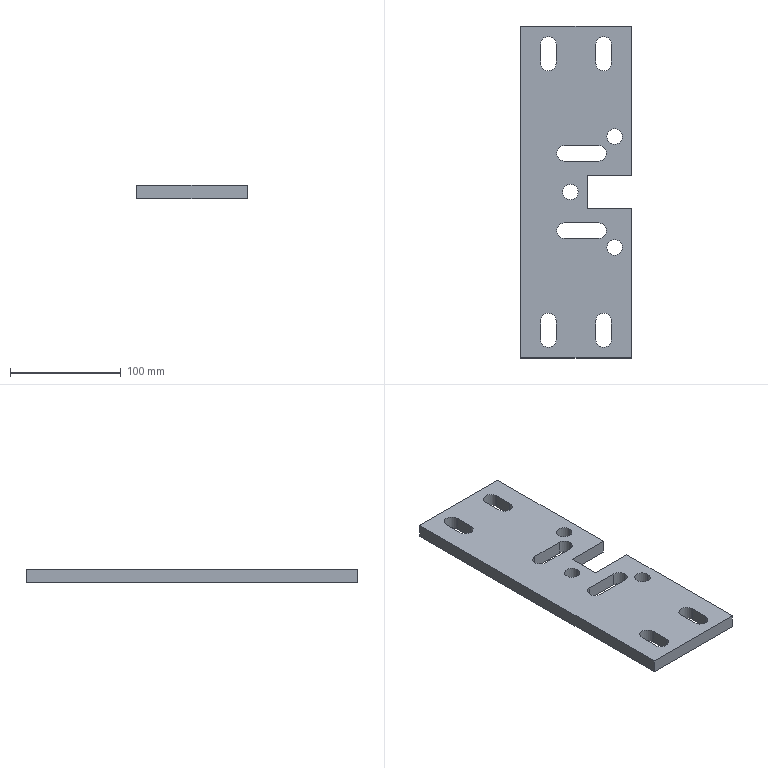Part | 1 solid | 42 faces | box 100 x 300 x 12 mm | volume 307135 mm3 | plane 22 | cylinder 20 | commonest cylinder face diameters 14 x20
STEP:
#1=CARTESIAN_POINT('',(28.,-50.,-12.));
#2=VERTEX_POINT('',#1);
#3=CARTESIAN_POINT('',(42.,-50.,-12.));
#4=VERTEX_POINT('',#3);
#5=CARTESIAN_POINT('',(35.,-50.,-12.));
#6=DIRECTION('',(0.,0.,1.));
#7=DIRECTION('',(1.,0.,0.));
#8=AXIS2_PLACEMENT_3D('',#5,#6,#7);
#9=CIRCLE('',#8,7.);
#10=EDGE_CURVE('',#2,#4,#9,.T.);
#11=ORIENTED_EDGE('',*,*,#10,.F.);
#12=CARTESIAN_POINT('',(28.,-50.,0.));
#13=VERTEX_POINT('',#12);
#14=CARTESIAN_POINT('',(28.,-50.,-12.));
#15=DIRECTION('',(0.,0.,1.));
#16=VECTOR('',#15,1000.);
#17=LINE('',#14,#16);
#18=EDGE_CURVE('',#2,#13,#17,.T.);
#19=ORIENTED_EDGE('',*,*,#18,.T.);
#20=CARTESIAN_POINT('',(42.,-50.,0.));
#21=VERTEX_POINT('',#20);
#22=CARTESIAN_POINT('',(35.,-50.,0.));
#23=DIRECTION('',(0.,0.,1.));
#24=DIRECTION('',(1.,0.,0.));
#25=AXIS2_PLACEMENT_3D('',#22,#23,#24);
#26=CIRCLE('',#25,7.);
#27=EDGE_CURVE('',#13,#21,#26,.T.);
#28=ORIENTED_EDGE('',*,*,#27,.T.);
#29=CARTESIAN_POINT('',(42.,-50.,-12.));
#30=DIRECTION('',(0.,0.,1.));
#31=VECTOR('',#30,1000.);
#32=LINE('',#29,#31);
#33=EDGE_CURVE('',#4,#21,#32,.T.);
#34=ORIENTED_EDGE('',*,*,#33,.F.);
#35=EDGE_LOOP('',(#11,#19,#28,#34));
#36=FACE_OUTER_BOUND('',#35,.T.);
#37=CARTESIAN_POINT('',(35.,-50.,-12.));
#38=DIRECTION('',(0.,0.,1.));
#39=DIRECTION('',(1.,0.,0.));
#40=AXIS2_PLACEMENT_3D('',#37,#38,#39);
#41=CYLINDRICAL_SURFACE('',#40,7.);
#42=ADVANCED_FACE('',(#36),#41,.F.);
#43=CARTESIAN_POINT('',(-12.,0.,-12.));
#44=VERTEX_POINT('',#43);
#45=CARTESIAN_POINT('',(2.,0.,-12.));
#46=VERTEX_POINT('',#45);
#47=CARTESIAN_POINT('',(-5.,0.,-12.));
#48=DIRECTION('',(0.,0.,1.));
#49=DIRECTION('',(1.,0.,0.));
#50=AXIS2_PLACEMENT_3D('',#47,#48,#49);
#51=CIRCLE('',#50,7.);
#52=EDGE_CURVE('',#44,#46,#51,.T.);
#53=ORIENTED_EDGE('',*,*,#52,.F.);
#54=CARTESIAN_POINT('',(-12.,0.,0.));
#55=VERTEX_POINT('',#54);
#56=CARTESIAN_POINT('',(-12.,0.,-12.));
#57=DIRECTION('',(0.,0.,1.));
#58=VECTOR('',#57,1000.);
#59=LINE('',#56,#58);
#60=EDGE_CURVE('',#44,#55,#59,.T.);
#61=ORIENTED_EDGE('',*,*,#60,.T.);
#62=CARTESIAN_POINT('',(2.,0.,0.));
#63=VERTEX_POINT('',#62);
#64=CARTESIAN_POINT('',(-5.,0.,0.));
#65=DIRECTION('',(0.,0.,1.));
#66=DIRECTION('',(1.,0.,0.));
#67=AXIS2_PLACEMENT_3D('',#64,#65,#66);
#68=CIRCLE('',#67,7.);
#69=EDGE_CURVE('',#55,#63,#68,.T.);
#70=ORIENTED_EDGE('',*,*,#69,.T.);
#71=CARTESIAN_POINT('',(2.,0.,-12.));
#72=DIRECTION('',(0.,0.,1.));
#73=VECTOR('',#72,1000.);
#74=LINE('',#71,#73);
#75=EDGE_CURVE('',#46,#63,#74,.T.);
#76=ORIENTED_EDGE('',*,*,#75,.F.);
#77=EDGE_LOOP('',(#53,#61,#70,#76));
#78=FACE_OUTER_BOUND('',#77,.T.);
#79=CARTESIAN_POINT('',(-5.,0.,-12.));
#80=DIRECTION('',(0.,0.,1.));
#81=DIRECTION('',(1.,0.,0.));
#82=AXIS2_PLACEMENT_3D('',#79,#80,#81);
#83=CYLINDRICAL_SURFACE('',#82,7.);
#84=ADVANCED_FACE('',(#78),#83,.F.);
#85=CARTESIAN_POINT('',(28.,50.,-12.));
#86=VERTEX_POINT('',#85);
#87=CARTESIAN_POINT('',(42.,50.,-12.));
#88=VERTEX_POINT('',#87);
#89=CARTESIAN_POINT('',(35.,50.,-12.));
#90=DIRECTION('',(0.,0.,1.));
#91=DIRECTION('',(-1.,0.,0.));
#92=AXIS2_PLACEMENT_3D('',#89,#90,#91);
#93=CIRCLE('',#92,7.);
#94=EDGE_CURVE('',#86,#88,#93,.T.);
#95=ORIENTED_EDGE('',*,*,#94,.F.);
#96=CARTESIAN_POINT('',(28.,50.,0.));
#97=VERTEX_POINT('',#96);
#98=CARTESIAN_POINT('',(28.,50.,-12.));
#99=DIRECTION('',(0.,0.,1.));
#100=VECTOR('',#99,1000.);
#101=LINE('',#98,#100);
#102=EDGE_CURVE('',#86,#97,#101,.T.);
#103=ORIENTED_EDGE('',*,*,#102,.T.);
#104=CARTESIAN_POINT('',(42.,50.,0.));
#105=VERTEX_POINT('',#104);
#106=CARTESIAN_POINT('',(35.,50.,0.));
#107=DIRECTION('',(0.,0.,1.));
#108=DIRECTION('',(1.,0.,0.));
#109=AXIS2_PLACEMENT_3D('',#106,#107,#108);
#110=CIRCLE('',#109,7.);
#111=EDGE_CURVE('',#97,#105,#110,.T.);
#112=ORIENTED_EDGE('',*,*,#111,.T.);
#113=CARTESIAN_POINT('',(42.,50.,-12.));
#114=DIRECTION('',(0.,0.,1.));
#115=VECTOR('',#114,1000.);
#116=LINE('',#113,#115);
#117=EDGE_CURVE('',#88,#105,#116,.T.);
#118=ORIENTED_EDGE('',*,*,#117,.F.);
#119=EDGE_LOOP('',(#95,#103,#112,#118));
#120=FACE_OUTER_BOUND('',#119,.T.);
#121=CARTESIAN_POINT('',(35.,50.,-12.));
#122=DIRECTION('',(0.,0.,1.));
#123=DIRECTION('',(1.,0.,0.));
#124=AXIS2_PLACEMENT_3D('',#121,#122,#123);
#125=CYLINDRICAL_SURFACE('',#124,7.);
#126=ADVANCED_FACE('',(#120),#125,.F.);
#127=CARTESIAN_POINT('',(27.5,-35.,-12.));
#128=VERTEX_POINT('',#127);
#129=CARTESIAN_POINT('',(20.5,-28.,-12.));
#130=VERTEX_POINT('',#129);
#131=CARTESIAN_POINT('',(20.5,-35.,-12.));
#132=DIRECTION('',(0.,0.,1.));
#133=DIRECTION('',(1.,0.,0.));
#134=AXIS2_PLACEMENT_3D('',#131,#132,#133);
#135=CIRCLE('',#134,7.);
#136=EDGE_CURVE('',#128,#130,#135,.T.);
#137=ORIENTED_EDGE('',*,*,#136,.F.);
#138=CARTESIAN_POINT('',(27.5,-35.,0.));
#139=VERTEX_POINT('',#138);
#140=CARTESIAN_POINT('',(27.5,-35.,-12.));
#141=DIRECTION('',(0.,0.,1.));
#142=VECTOR('',#141,1000.);
#143=LINE('',#140,#142);
#144=EDGE_CURVE('',#128,#139,#143,.T.);
#145=ORIENTED_EDGE('',*,*,#144,.T.);
#146=CARTESIAN_POINT('',(20.5,-28.,0.));
#147=VERTEX_POINT('',#146);
#148=CARTESIAN_POINT('',(20.5,-35.,0.));
#149=DIRECTION('',(0.,0.,1.));
#150=DIRECTION('',(1.,0.,0.));
#151=AXIS2_PLACEMENT_3D('',#148,#149,#150);
#152=CIRCLE('',#151,7.);
#153=EDGE_CURVE('',#139,#147,#152,.T.);
#154=ORIENTED_EDGE('',*,*,#153,.T.);
#155=CARTESIAN_POINT('',(20.5,-28.,-12.));
#156=DIRECTION('',(0.,0.,1.));
#157=VECTOR('',#156,1000.);
#158=LINE('',#155,#157);
#159=EDGE_CURVE('',#130,#147,#158,.T.);
#160=ORIENTED_EDGE('',*,*,#159,.F.);
#161=EDGE_LOOP('',(#137,#145,#154,#160));
#162=FACE_OUTER_BOUND('',#161,.T.);
#163=CARTESIAN_POINT('',(20.5,-35.,-12.));
#164=DIRECTION('',(0.,0.,1.));
#165=DIRECTION('',(1.,0.,0.));
#166=AXIS2_PLACEMENT_3D('',#163,#164,#165);
#167=CYLINDRICAL_SURFACE('',#166,7.);
#168=ADVANCED_FACE('',(#162),#167,.F.);
#169=CARTESIAN_POINT('',(27.5,35.,-12.));
#170=VERTEX_POINT('',#169);
#171=CARTESIAN_POINT('',(20.5,42.,-12.));
#172=VERTEX_POINT('',#171);
#173=CARTESIAN_POINT('',(20.5,35.,-12.));
#174=DIRECTION('',(0.,0.,1.));
#175=DIRECTION('',(-1.,0.,0.));
#176=AXIS2_PLACEMENT_3D('',#173,#174,#175);
#177=CIRCLE('',#176,7.);
#178=EDGE_CURVE('',#170,#172,#177,.T.);
#179=ORIENTED_EDGE('',*,*,#178,.F.);
#180=CARTESIAN_POINT('',(27.5,35.,0.));
#181=VERTEX_POINT('',#180);
#182=CARTESIAN_POINT('',(27.5,35.,-12.));
#183=DIRECTION('',(0.,0.,1.));
#184=VECTOR('',#183,1000.);
#185=LINE('',#182,#184);
#186=EDGE_CURVE('',#170,#181,#185,.T.);
#187=ORIENTED_EDGE('',*,*,#186,.T.);
#188=CARTESIAN_POINT('',(20.5,42.,0.));
#189=VERTEX_POINT('',#188);
#190=CARTESIAN_POINT('',(20.5,35.,0.));
#191=DIRECTION('',(0.,0.,1.));
#192=DIRECTION('',(1.,0.,0.));
#193=AXIS2_PLACEMENT_3D('',#190,#191,#192);
#194=CIRCLE('',#193,7.);
#195=EDGE_CURVE('',#181,#189,#194,.T.);
#196=ORIENTED_EDGE('',*,*,#195,.T.);
#197=CARTESIAN_POINT('',(20.5,42.,-12.));
#198=DIRECTION('',(0.,0.,1.));
#199=VECTOR('',#198,1000.);
#200=LINE('',#197,#199);
#201=EDGE_CURVE('',#172,#189,#200,.T.);
#202=ORIENTED_EDGE('',*,*,#201,.F.);
#203=EDGE_LOOP('',(#179,#187,#196,#202));
#204=FACE_OUTER_BOUND('',#203,.T.);
#205=CARTESIAN_POINT('',(20.5,35.,-12.));
#206=DIRECTION('',(0.,0.,1.));
#207=DIRECTION('',(1.,0.,0.));
#208=AXIS2_PLACEMENT_3D('',#205,#206,#207);
#209=CYLINDRICAL_SURFACE('',#208,7.);
#210=ADVANCED_FACE('',(#204),#209,.F.);
#211=CARTESIAN_POINT('',(50.,-15.,0.));
#212=VERTEX_POINT('',#211);
#213=CARTESIAN_POINT('',(50.,-15.,-12.));
#214=VERTEX_POINT('',#213);
#215=CARTESIAN_POINT('',(50.,-15.,-12.));
#216=DIRECTION('',(0.,0.,-1.));
#217=VECTOR('',#216,1000.);
#218=LINE('',#215,#217);
#219=EDGE_CURVE('',#212,#214,#218,.T.);
#220=ORIENTED_EDGE('',*,*,#219,.F.);
#221=CARTESIAN_POINT('',(50.,-150.,0.));
#222=VERTEX_POINT('',#221);
#223=CARTESIAN_POINT('',(50.,150.,0.));
#224=DIRECTION('',(0.,1.,0.));
#225=VECTOR('',#224,1000.);
#226=LINE('',#223,#225);
#227=EDGE_CURVE('',#222,#212,#226,.T.);
#228=ORIENTED_EDGE('',*,*,#227,.F.);
#229=CARTESIAN_POINT('',(50.,-150.,-12.));
#230=VERTEX_POINT('',#229);
#231=CARTESIAN_POINT('',(50.,-150.,-12.));
#232=DIRECTION('',(0.,0.,1.));
#233=VECTOR('',#232,1000.);
#234=LINE('',#231,#233);
#235=EDGE_CURVE('',#230,#222,#234,.T.);
#236=ORIENTED_EDGE('',*,*,#235,.F.);
#237=CARTESIAN_POINT('',(50.,150.,-12.));
#238=DIRECTION('',(0.,1.,0.));
#239=VECTOR('',#238,1000.);
#240=LINE('',#237,#239);
#241=EDGE_CURVE('',#230,#214,#240,.T.);
#242=ORIENTED_EDGE('',*,*,#241,.T.);
#243=EDGE_LOOP('',(#220,#228,#236,#242));
#244=FACE_OUTER_BOUND('',#243,.T.);
#245=CARTESIAN_POINT('',(50.,150.,-12.));
#246=DIRECTION('',(1.,0.,0.));
#247=DIRECTION('',(0.,1.,0.));
#248=AXIS2_PLACEMENT_3D('',#245,#246,#247);
#249=PLANE('',#248);
#250=ADVANCED_FACE('',(#244),#249,.T.);
#251=CARTESIAN_POINT('',(50.,15.,-12.));
#252=VERTEX_POINT('',#251);
#253=CARTESIAN_POINT('',(50.,15.,0.));
#254=VERTEX_POINT('',#253);
#255=CARTESIAN_POINT('',(50.,15.,-12.));
#256=DIRECTION('',(0.,0.,1.));
#257=VECTOR('',#256,1000.);
#258=LINE('',#255,#257);
#259=EDGE_CURVE('',#252,#254,#258,.T.);
#260=ORIENTED_EDGE('',*,*,#259,.F.);
#261=CARTESIAN_POINT('',(50.,150.,-12.));
#262=VERTEX_POINT('',#261);
#263=CARTESIAN_POINT('',(50.,150.,-12.));
#264=DIRECTION('',(0.,1.,0.));
#265=VECTOR('',#264,1000.);
#266=LINE('',#263,#265);
#267=EDGE_CURVE('',#252,#262,#266,.T.);
#268=ORIENTED_EDGE('',*,*,#267,.T.);
#269=CARTESIAN_POINT('',(50.,150.,0.));
#270=VERTEX_POINT('',#269);
#271=CARTESIAN_POINT('',(50.,150.,-12.));
#272=DIRECTION('',(0.,0.,1.));
#273=VECTOR('',#272,1000.);
#274=LINE('',#271,#273);
#275=EDGE_CURVE('',#262,#270,#274,.T.);
#276=ORIENTED_EDGE('',*,*,#275,.T.);
#277=CARTESIAN_POINT('',(50.,150.,0.));
#278=DIRECTION('',(0.,1.,0.));
#279=VECTOR('',#278,1000.);
#280=LINE('',#277,#279);
#281=EDGE_CURVE('',#254,#270,#280,.T.);
#282=ORIENTED_EDGE('',*,*,#281,.F.);
#283=EDGE_LOOP('',(#260,#268,#276,#282));
#284=FACE_OUTER_BOUND('',#283,.T.);
#285=CARTESIAN_POINT('',(50.,150.,-12.));
#286=DIRECTION('',(1.,0.,0.));
#287=DIRECTION('',(0.,1.,0.));
#288=AXIS2_PLACEMENT_3D('',#285,#286,#287);
#289=PLANE('',#288);
#290=ADVANCED_FACE('',(#284),#289,.T.);
#291=CARTESIAN_POINT('',(-50.,-150.,0.));
#292=VERTEX_POINT('',#291);
#293=CARTESIAN_POINT('',(-50.,-150.,0.));
#294=DIRECTION('',(1.,0.,0.));
#295=VECTOR('',#294,1000.);
#296=LINE('',#293,#295);
#297=EDGE_CURVE('',#292,#222,#296,.T.);
#298=ORIENTED_EDGE('',*,*,#297,.F.);
#299=CARTESIAN_POINT('',(-50.,-150.,-12.));
#300=VERTEX_POINT('',#299);
#301=CARTESIAN_POINT('',(-50.,-150.,-12.));
#302=DIRECTION('',(0.,0.,1.));
#303=VECTOR('',#302,1000.);
#304=LINE('',#301,#303);
#305=EDGE_CURVE('',#300,#292,#304,.T.);
#306=ORIENTED_EDGE('',*,*,#305,.F.);
#307=CARTESIAN_POINT('',(-50.,-150.,-12.));
#308=DIRECTION('',(1.,0.,0.));
#309=VECTOR('',#308,1000.);
#310=LINE('',#307,#309);
#311=EDGE_CURVE('',#300,#230,#310,.T.);
#312=ORIENTED_EDGE('',*,*,#311,.T.);
#313=ORIENTED_EDGE('',*,*,#235,.T.);
#314=EDGE_LOOP('',(#298,#306,#312,#313));
#315=FACE_OUTER_BOUND('',#314,.T.);
#316=CARTESIAN_POINT('',(-50.,-150.,-12.));
#317=DIRECTION('',(0.,-1.,0.));
#318=DIRECTION('',(0.,0.,-1.));
#319=AXIS2_PLACEMENT_3D('',#316,#317,#318);
#320=PLANE('',#319);
#321=ADVANCED_FACE('',(#315),#320,.T.);
#322=CARTESIAN_POINT('',(-50.,150.,0.));
#323=VERTEX_POINT('',#322);
#324=CARTESIAN_POINT('',(-50.,150.,0.));
#325=DIRECTION('',(0.,-1.,0.));
#326=VECTOR('',#325,1000.);
#327=LINE('',#324,#326);
#328=EDGE_CURVE('',#323,#292,#327,.T.);
#329=ORIENTED_EDGE('',*,*,#328,.F.);
#330=CARTESIAN_POINT('',(-50.,150.,-12.));
#331=VERTEX_POINT('',#330);
#332=CARTESIAN_POINT('',(-50.,150.,-12.));
#333=DIRECTION('',(0.,0.,1.));
#334=VECTOR('',#333,1000.);
#335=LINE('',#332,#334);
#336=EDGE_CURVE('',#331,#323,#335,.T.);
#337=ORIENTED_EDGE('',*,*,#336,.F.);
#338=CARTESIAN_POINT('',(-50.,150.,-12.));
#339=DIRECTION('',(0.,-1.,0.));
#340=VECTOR('',#339,1000.);
#341=LINE('',#338,#340);
#342=EDGE_CURVE('',#331,#300,#341,.T.);
#343=ORIENTED_EDGE('',*,*,#342,.T.);
#344=ORIENTED_EDGE('',*,*,#305,.T.);
#345=EDGE_LOOP('',(#329,#337,#343,#344));
#346=FACE_OUTER_BOUND('',#345,.T.);
#347=CARTESIAN_POINT('',(-50.,150.,-12.));
#348=DIRECTION('',(-1.,0.,0.));
#349=DIRECTION('',(0.,-1.,0.));
#350=AXIS2_PLACEMENT_3D('',#347,#348,#349);
#351=PLANE('',#350);
#352=ADVANCED_FACE('',(#346),#351,.T.);
#353=CARTESIAN_POINT('',(-50.,150.,0.));
#354=DIRECTION('',(-1.,0.,0.));
#355=VECTOR('',#354,1000.);
#356=LINE('',#353,#355);
#357=EDGE_CURVE('',#270,#323,#356,.T.);
#358=ORIENTED_EDGE('',*,*,#357,.F.);
#359=ORIENTED_EDGE('',*,*,#275,.F.);
#360=CARTESIAN_POINT('',(-50.,150.,-12.));
#361=DIRECTION('',(-1.,0.,0.));
#362=VECTOR('',#361,1000.);
#363=LINE('',#360,#362);
#364=EDGE_CURVE('',#262,#331,#363,.T.);
#365=ORIENTED_EDGE('',*,*,#364,.T.);
#366=ORIENTED_EDGE('',*,*,#336,.T.);
#367=EDGE_LOOP('',(#358,#359,#365,#366));
#368=FACE_OUTER_BOUND('',#367,.T.);
#369=CARTESIAN_POINT('',(-50.,150.,-12.));
#370=DIRECTION('',(0.,1.,0.));
#371=DIRECTION('',(0.,0.,1.));
#372=AXIS2_PLACEMENT_3D('',#369,#370,#371);
#373=PLANE('',#372);
#374=ADVANCED_FACE('',(#368),#373,.T.);
#375=CARTESIAN_POINT('',(35.,-50.,-12.));
#376=DIRECTION('',(0.,0.,1.));
#377=DIRECTION('',(1.,0.,0.));
#378=AXIS2_PLACEMENT_3D('',#375,#376,#377);
#379=CIRCLE('',#378,7.);
#380=EDGE_CURVE('',#4,#2,#379,.T.);
#381=ORIENTED_EDGE('',*,*,#380,.T.);
#382=ORIENTED_EDGE('',*,*,#10,.T.);
#383=EDGE_LOOP('',(#381,#382));
#384=FACE_BOUND('',#383,.T.);
#385=CARTESIAN_POINT('',(-5.,0.,-12.));
#386=DIRECTION('',(0.,0.,1.));
#387=DIRECTION('',(1.,0.,0.));
#388=AXIS2_PLACEMENT_3D('',#385,#386,#387);
#389=CIRCLE('',#388,7.);
#390=EDGE_CURVE('',#46,#44,#389,.T.);
#391=ORIENTED_EDGE('',*,*,#390,.T.);
#392=ORIENTED_EDGE('',*,*,#52,.T.);
#393=EDGE_LOOP('',(#391,#392));
#394=FACE_BOUND('',#393,.T.);
#395=CARTESIAN_POINT('',(35.,50.,-12.));
#396=DIRECTION('',(0.,0.,1.));
#397=DIRECTION('',(-1.,0.,0.));
#398=AXIS2_PLACEMENT_3D('',#395,#396,#397);
#399=CIRCLE('',#398,7.);
#400=EDGE_CURVE('',#88,#86,#399,.T.);
#401=ORIENTED_EDGE('',*,*,#400,.T.);
#402=ORIENTED_EDGE('',*,*,#94,.T.);
#403=EDGE_LOOP('',(#401,#402));
#404=FACE_BOUND('',#403,.T.);
#405=CARTESIAN_POINT('',(-10.5,-28.,-12.));
#406=VERTEX_POINT('',#405);
#407=CARTESIAN_POINT('',(-10.5,-28.,-12.));
#408=DIRECTION('',(-1.,0.,0.));
#409=VECTOR('',#408,1000.);
#410=LINE('',#407,#409);
#411=EDGE_CURVE('',#130,#406,#410,.T.);
#412=ORIENTED_EDGE('',*,*,#411,.T.);
#413=CARTESIAN_POINT('',(-10.5,-42.,-12.));
#414=VERTEX_POINT('',#413);
#415=CARTESIAN_POINT('',(-10.5,-35.,-12.));
#416=DIRECTION('',(0.,0.,1.));
#417=DIRECTION('',(1.,0.,0.));
#418=AXIS2_PLACEMENT_3D('',#415,#416,#417);
#419=CIRCLE('',#418,7.);
#420=EDGE_CURVE('',#406,#414,#419,.T.);
#421=ORIENTED_EDGE('',*,*,#420,.T.);
#422=CARTESIAN_POINT('',(20.5,-42.,-12.));
#423=VERTEX_POINT('',#422);
#424=CARTESIAN_POINT('',(-10.5,-42.,-12.));
#425=DIRECTION('',(1.,0.,0.));
#426=VECTOR('',#425,1000.);
#427=LINE('',#424,#426);
#428=EDGE_CURVE('',#414,#423,#427,.T.);
#429=ORIENTED_EDGE('',*,*,#428,.T.);
#430=CARTESIAN_POINT('',(20.5,-35.,-12.));
#431=DIRECTION('',(0.,0.,1.));
#432=DIRECTION('',(1.,0.,0.));
#433=AXIS2_PLACEMENT_3D('',#430,#431,#432);
#434=CIRCLE('',#433,7.);
#435=EDGE_CURVE('',#423,#128,#434,.T.);
#436=ORIENTED_EDGE('',*,*,#435,.T.);
#437=ORIENTED_EDGE('',*,*,#136,.T.);
#438=EDGE_LOOP('',(#412,#421,#429,#436,#437));
#439=FACE_BOUND('',#438,.T.);
#440=CARTESIAN_POINT('',(-18.,116.5,-12.));
#441=VERTEX_POINT('',#440);
#442=CARTESIAN_POINT('',(-18.,133.5,-12.));
#443=VERTEX_POINT('',#442);
#444=CARTESIAN_POINT('',(-18.,133.5,-12.));
#445=DIRECTION('',(0.,1.,0.));
#446=VECTOR('',#445,1000.);
#447=LINE('',#444,#446);
#448=EDGE_CURVE('',#441,#443,#447,.T.);
#449=ORIENTED_EDGE('',*,*,#448,.T.);
#450=CARTESIAN_POINT('',(-32.,133.5,-12.));
#451=VERTEX_POINT('',#450);
#452=CARTESIAN_POINT('',(-25.,133.5,-12.));
#453=DIRECTION('',(0.,0.,1.));
#454=DIRECTION('',(-1.,0.,0.));
#455=AXIS2_PLACEMENT_3D('',#452,#453,#454);
#456=CIRCLE('',#455,7.);
#457=EDGE_CURVE('',#443,#451,#456,.T.);
#458=ORIENTED_EDGE('',*,*,#457,.T.);
#459=CARTESIAN_POINT('',(-32.,116.5,-12.));
#460=VERTEX_POINT('',#459);
#461=CARTESIAN_POINT('',(-32.,133.5,-12.));
#462=DIRECTION('',(0.,-1.,0.));
#463=VECTOR('',#462,1000.);
#464=LINE('',#461,#463);
#465=EDGE_CURVE('',#451,#460,#464,.T.);
#466=ORIENTED_EDGE('',*,*,#465,.T.);
#467=CARTESIAN_POINT('',(-25.,116.5,-12.));
#468=DIRECTION('',(0.,0.,1.));
#469=DIRECTION('',(-1.,0.,0.));
#470=AXIS2_PLACEMENT_3D('',#467,#468,#469);
#471=CIRCLE('',#470,7.);
#472=EDGE_CURVE('',#460,#441,#471,.T.);
#473=ORIENTED_EDGE('',*,*,#472,.T.);
#474=EDGE_LOOP('',(#449,#458,#466,#473));
#475=FACE_BOUND('',#474,.T.);
#476=CARTESIAN_POINT('',(32.,116.5,-12.));
#477=VERTEX_POINT('',#476);
#478=CARTESIAN_POINT('',(32.,133.5,-12.));
#479=VERTEX_POINT('',#478);
#480=CARTESIAN_POINT('',(32.,133.5,-12.));
#481=DIRECTION('',(0.,1.,0.));
#482=VECTOR('',#481,1000.);
#483=LINE('',#480,#482);
#484=EDGE_CURVE('',#477,#479,#483,.T.);
#485=ORIENTED_EDGE('',*,*,#484,.T.);
#486=CARTESIAN_POINT('',(18.,133.5,-12.));
#487=VERTEX_POINT('',#486);
#488=CARTESIAN_POINT('',(25.,133.5,-12.));
#489=DIRECTION('',(0.,0.,1.));
#490=DIRECTION('',(-1.,0.,0.));
#491=AXIS2_PLACEMENT_3D('',#488,#489,#490);
#492=CIRCLE('',#491,7.);
#493=EDGE_CURVE('',#479,#487,#492,.T.);
#494=ORIENTED_EDGE('',*,*,#493,.T.);
#495=CARTESIAN_POINT('',(18.,116.5,-12.));
#496=VERTEX_POINT('',#495);
#497=CARTESIAN_POINT('',(18.,133.5,-12.));
#498=DIRECTION('',(0.,-1.,0.));
#499=VECTOR('',#498,1000.);
#500=LINE('',#497,#499);
#501=EDGE_CURVE('',#487,#496,#500,.T.);
#502=ORIENTED_EDGE('',*,*,#501,.T.);
#503=CARTESIAN_POINT('',(25.,116.5,-12.));
#504=DIRECTION('',(0.,0.,1.));
#505=DIRECTION('',(-1.,0.,0.));
#506=AXIS2_PLACEMENT_3D('',#503,#504,#505);
#507=CIRCLE('',#506,7.);
#508=EDGE_CURVE('',#496,#477,#507,.T.);
#509=ORIENTED_EDGE('',*,*,#508,.T.);
#510=EDGE_LOOP('',(#485,#494,#502,#509));
#511=FACE_BOUND('',#510,.T.);
#512=CARTESIAN_POINT('',(18.,-116.5,-12.));
#513=VERTEX_POINT('',#512);
#514=CARTESIAN_POINT('',(18.,-133.5,-12.));
#515=VERTEX_POINT('',#514);
#516=CARTESIAN_POINT('',(18.,-133.5,-12.));
#517=DIRECTION('',(0.,-1.,0.));
#518=VECTOR('',#517,1000.);
#519=LINE('',#516,#518);
#520=EDGE_CURVE('',#513,#515,#519,.T.);
#521=ORIENTED_EDGE('',*,*,#520,.T.);
#522=CARTESIAN_POINT('',(32.,-133.5,-12.));
#523=VERTEX_POINT('',#522);
#524=CARTESIAN_POINT('',(25.,-133.5,-12.));
#525=DIRECTION('',(0.,0.,1.));
#526=DIRECTION('',(1.,0.,0.));
#527=AXIS2_PLACEMENT_3D('',#524,#525,#526);
#528=CIRCLE('',#527,7.);
#529=EDGE_CURVE('',#515,#523,#528,.T.);
#530=ORIENTED_EDGE('',*,*,#529,.T.);
#531=CARTESIAN_POINT('',(32.,-116.5,-12.));
#532=VERTEX_POINT('',#531);
#533=CARTESIAN_POINT('',(32.,-133.5,-12.));
#534=DIRECTION('',(0.,1.,0.));
#535=VECTOR('',#534,1000.);
#536=LINE('',#533,#535);
#537=EDGE_CURVE('',#523,#532,#536,.T.);
#538=ORIENTED_EDGE('',*,*,#537,.T.);
#539=CARTESIAN_POINT('',(25.,-116.5,-12.));
#540=DIRECTION('',(0.,0.,1.));
#541=DIRECTION('',(1.,0.,0.));
#542=AXIS2_PLACEMENT_3D('',#539,#540,#541);
#543=CIRCLE('',#542,7.);
#544=EDGE_CURVE('',#532,#513,#543,.T.);
#545=ORIENTED_EDGE('',*,*,#544,.T.);
#546=EDGE_LOOP('',(#521,#530,#538,#545));
#547=FACE_BOUND('',#546,.T.);
#548=CARTESIAN_POINT('',(-32.,-116.5,-12.));
#549=VERTEX_POINT('',#548);
#550=CARTESIAN_POINT('',(-32.,-133.5,-12.));
#551=VERTEX_POINT('',#550);
#552=CARTESIAN_POINT('',(-32.,-133.5,-12.));
#553=DIRECTION('',(0.,-1.,0.));
#554=VECTOR('',#553,1000.);
#555=LINE('',#552,#554);
#556=EDGE_CURVE('',#549,#551,#555,.T.);
#557=ORIENTED_EDGE('',*,*,#556,.T.);
#558=CARTESIAN_POINT('',(-18.,-133.5,-12.));
#559=VERTEX_POINT('',#558);
#560=CARTESIAN_POINT('',(-25.,-133.5,-12.));
#561=DIRECTION('',(0.,0.,1.));
#562=DIRECTION('',(1.,0.,0.));
#563=AXIS2_PLACEMENT_3D('',#560,#561,#562);
#564=CIRCLE('',#563,7.);
#565=EDGE_CURVE('',#551,#559,#564,.T.);
#566=ORIENTED_EDGE('',*,*,#565,.T.);
#567=CARTESIAN_POINT('',(-18.,-116.5,-12.));
#568=VERTEX_POINT('',#567);
#569=CARTESIAN_POINT('',(-18.,-133.5,-12.));
#570=DIRECTION('',(0.,1.,0.));
#571=VECTOR('',#570,1000.);
#572=LINE('',#569,#571);
#573=EDGE_CURVE('',#559,#568,#572,.T.);
#574=ORIENTED_EDGE('',*,*,#573,.T.);
#575=CARTESIAN_POINT('',(-25.,-116.5,-12.));
#576=DIRECTION('',(0.,0.,1.));
#577=DIRECTION('',(1.,0.,0.));
#578=AXIS2_PLACEMENT_3D('',#575,#576,#577);
#579=CIRCLE('',#578,7.);
#580=EDGE_CURVE('',#568,#549,#579,.T.);
#581=ORIENTED_EDGE('',*,*,#580,.T.);
#582=EDGE_LOOP('',(#557,#566,#574,#581));
#583=FACE_BOUND('',#582,.T.);
#584=CARTESIAN_POINT('',(-10.5,42.,-12.));
#585=VERTEX_POINT('',#584);
#586=CARTESIAN_POINT('',(-10.5,42.,-12.));
#587=DIRECTION('',(-1.,0.,0.));
#588=VECTOR('',#587,1000.);
#589=LINE('',#586,#588);
#590=EDGE_CURVE('',#172,#585,#589,.T.);
#591=ORIENTED_EDGE('',*,*,#590,.T.);
#592=CARTESIAN_POINT('',(-10.5,28.,-12.));
#593=VERTEX_POINT('',#592);
#594=CARTESIAN_POINT('',(-10.5,35.,-12.));
#595=DIRECTION('',(0.,0.,1.));
#596=DIRECTION('',(-1.,0.,0.));
#597=AXIS2_PLACEMENT_3D('',#594,#595,#596);
#598=CIRCLE('',#597,7.);
#599=EDGE_CURVE('',#585,#593,#598,.T.);
#600=ORIENTED_EDGE('',*,*,#599,.T.);
#601=CARTESIAN_POINT('',(20.5,28.,-12.));
#602=VERTEX_POINT('',#601);
#603=CARTESIAN_POINT('',(-10.5,28.,-12.));
#604=DIRECTION('',(1.,0.,0.));
#605=VECTOR('',#604,1000.);
#606=LINE('',#603,#605);
#607=EDGE_CURVE('',#593,#602,#606,.T.);
#608=ORIENTED_EDGE('',*,*,#607,.T.);
#609=CARTESIAN_POINT('',(20.5,35.,-12.));
#610=DIRECTION('',(0.,0.,1.));
#611=DIRECTION('',(-1.,0.,0.));
#612=AXIS2_PLACEMENT_3D('',#609,#610,#611);
#613=CIRCLE('',#612,7.);
#614=EDGE_CURVE('',#602,#170,#613,.T.);
#615=ORIENTED_EDGE('',*,*,#614,.T.);
#616=ORIENTED_EDGE('',*,*,#178,.T.);
#617=EDGE_LOOP('',(#591,#600,#608,#615,#616));
#618=FACE_BOUND('',#617,.T.);
#619=CARTESIAN_POINT('',(10.,15.,-12.));
#620=VERTEX_POINT('',#619);
#621=CARTESIAN_POINT('',(10.,-15.,-12.));
#622=VERTEX_POINT('',#621);
#623=CARTESIAN_POINT('',(10.,-15.,-12.));
#624=DIRECTION('',(0.,-1.,0.));
#625=VECTOR('',#624,1000.);
#626=LINE('',#623,#625);
#627=EDGE_CURVE('',#620,#622,#626,.T.);
#628=ORIENTED_EDGE('',*,*,#627,.T.);
#629=CARTESIAN_POINT('',(10.,-15.,-12.));
#630=DIRECTION('',(1.,0.,0.));
#631=VECTOR('',#630,1000.);
#632=LINE('',#629,#631);
#633=EDGE_CURVE('',#622,#214,#632,.T.);
#634=ORIENTED_EDGE('',*,*,#633,.T.);
#635=ORIENTED_EDGE('',*,*,#241,.F.);
#636=ORIENTED_EDGE('',*,*,#311,.F.);
#637=ORIENTED_EDGE('',*,*,#342,.F.);
#638=ORIENTED_EDGE('',*,*,#364,.F.);
#639=ORIENTED_EDGE('',*,*,#267,.F.);
#640=CARTESIAN_POINT('',(10.,15.,-12.));
#641=DIRECTION('',(-1.,0.,0.));
#642=VECTOR('',#641,1000.);
#643=LINE('',#640,#642);
#644=EDGE_CURVE('',#252,#620,#643,.T.);
#645=ORIENTED_EDGE('',*,*,#644,.T.);
#646=EDGE_LOOP('',(#628,#634,#635,#636,#637,#638,#639,#645));
#647=FACE_OUTER_BOUND('',#646,.T.);
#648=CARTESIAN_POINT('',(0.,0.,-12.));
#649=DIRECTION('',(0.,0.,1.));
#650=DIRECTION('',(1.,0.,0.));
#651=AXIS2_PLACEMENT_3D('',#648,#649,#650);
#652=PLANE('',#651);
#653=ADVANCED_FACE('',(#384,#394,#404,#439,#475,#511,#547,#583,#618,#647),#652,.F.);
#654=CARTESIAN_POINT('',(35.,-50.,0.));
#655=DIRECTION('',(0.,0.,1.));
#656=DIRECTION('',(1.,0.,0.));
#657=AXIS2_PLACEMENT_3D('',#654,#655,#656);
#658=CIRCLE('',#657,7.);
#659=EDGE_CURVE('',#21,#13,#658,.T.);
#660=ORIENTED_EDGE('',*,*,#659,.F.);
#661=ORIENTED_EDGE('',*,*,#27,.F.);
#662=EDGE_LOOP('',(#660,#661));
#663=FACE_BOUND('',#662,.T.);
#664=CARTESIAN_POINT('',(-5.,0.,0.));
#665=DIRECTION('',(0.,0.,1.));
#666=DIRECTION('',(1.,0.,0.));
#667=AXIS2_PLACEMENT_3D('',#664,#665,#666);
#668=CIRCLE('',#667,7.);
#669=EDGE_CURVE('',#63,#55,#668,.T.);
#670=ORIENTED_EDGE('',*,*,#669,.F.);
#671=ORIENTED_EDGE('',*,*,#69,.F.);
#672=EDGE_LOOP('',(#670,#671));
#673=FACE_BOUND('',#672,.T.);
#674=CARTESIAN_POINT('',(35.,50.,0.));
#675=DIRECTION('',(0.,0.,1.));
#676=DIRECTION('',(1.,0.,0.));
#677=AXIS2_PLACEMENT_3D('',#674,#675,#676);
#678=CIRCLE('',#677,7.);
#679=EDGE_CURVE('',#105,#97,#678,.T.);
#680=ORIENTED_EDGE('',*,*,#679,.F.);
#681=ORIENTED_EDGE('',*,*,#111,.F.);
#682=EDGE_LOOP('',(#680,#681));
#683=FACE_BOUND('',#682,.T.);
#684=CARTESIAN_POINT('',(-10.5,-28.,0.));
#685=VERTEX_POINT('',#684);
#686=CARTESIAN_POINT('',(-10.5,-42.,0.));
#687=VERTEX_POINT('',#686);
#688=CARTESIAN_POINT('',(-10.5,-35.,0.));
#689=DIRECTION('',(0.,0.,1.));
#690=DIRECTION('',(1.,0.,0.));
#691=AXIS2_PLACEMENT_3D('',#688,#689,#690);
#692=CIRCLE('',#691,7.);
#693=EDGE_CURVE('',#685,#687,#692,.T.);
#694=ORIENTED_EDGE('',*,*,#693,.F.);
#695=CARTESIAN_POINT('',(-10.5,-28.,0.));
#696=DIRECTION('',(-1.,0.,0.));
#697=VECTOR('',#696,1000.);
#698=LINE('',#695,#697);
#699=EDGE_CURVE('',#147,#685,#698,.T.);
#700=ORIENTED_EDGE('',*,*,#699,.F.);
#701=ORIENTED_EDGE('',*,*,#153,.F.);
#702=CARTESIAN_POINT('',(20.5,-42.,0.));
#703=VERTEX_POINT('',#702);
#704=CARTESIAN_POINT('',(20.5,-35.,0.));
#705=DIRECTION('',(0.,0.,1.));
#706=DIRECTION('',(1.,0.,0.));
#707=AXIS2_PLACEMENT_3D('',#704,#705,#706);
#708=CIRCLE('',#707,7.);
#709=EDGE_CURVE('',#703,#139,#708,.T.);
#710=ORIENTED_EDGE('',*,*,#709,.F.);
#711=CARTESIAN_POINT('',(-10.5,-42.,0.));
#712=DIRECTION('',(1.,0.,0.));
#713=VECTOR('',#712,1000.);
#714=LINE('',#711,#713);
#715=EDGE_CURVE('',#687,#703,#714,.T.);
#716=ORIENTED_EDGE('',*,*,#715,.F.);
#717=EDGE_LOOP('',(#694,#700,#701,#710,#716));
#718=FACE_BOUND('',#717,.T.);
#719=CARTESIAN_POINT('',(-18.,133.5,0.));
#720=VERTEX_POINT('',#719);
#721=CARTESIAN_POINT('',(-32.,133.5,0.));
#722=VERTEX_POINT('',#721);
#723=CARTESIAN_POINT('',(-25.,133.5,0.));
#724=DIRECTION('',(0.,0.,1.));
#725=DIRECTION('',(1.,0.,0.));
#726=AXIS2_PLACEMENT_3D('',#723,#724,#725);
#727=CIRCLE('',#726,7.);
#728=EDGE_CURVE('',#720,#722,#727,.T.);
#729=ORIENTED_EDGE('',*,*,#728,.F.);
#730=CARTESIAN_POINT('',(-18.,116.5,0.));
#731=VERTEX_POINT('',#730);
#732=CARTESIAN_POINT('',(-18.,133.5,0.));
#733=DIRECTION('',(0.,1.,0.));
#734=VECTOR('',#733,1000.);
#735=LINE('',#732,#734);
#736=EDGE_CURVE('',#731,#720,#735,.T.);
#737=ORIENTED_EDGE('',*,*,#736,.F.);
#738=CARTESIAN_POINT('',(-32.,116.5,0.));
#739=VERTEX_POINT('',#738);
#740=CARTESIAN_POINT('',(-25.,116.5,0.));
#741=DIRECTION('',(0.,0.,1.));
#742=DIRECTION('',(1.,0.,0.));
#743=AXIS2_PLACEMENT_3D('',#740,#741,#742);
#744=CIRCLE('',#743,7.);
#745=EDGE_CURVE('',#739,#731,#744,.T.);
#746=ORIENTED_EDGE('',*,*,#745,.F.);
#747=CARTESIAN_POINT('',(-32.,133.5,0.));
#748=DIRECTION('',(0.,-1.,0.));
#749=VECTOR('',#748,1000.);
#750=LINE('',#747,#749);
#751=EDGE_CURVE('',#722,#739,#750,.T.);
#752=ORIENTED_EDGE('',*,*,#751,.F.);
#753=EDGE_LOOP('',(#729,#737,#746,#752));
#754=FACE_BOUND('',#753,.T.);
#755=CARTESIAN_POINT('',(32.,133.5,0.));
#756=VERTEX_POINT('',#755);
#757=CARTESIAN_POINT('',(18.,133.5,0.));
#758=VERTEX_POINT('',#757);
#759=CARTESIAN_POINT('',(25.,133.5,0.));
#760=DIRECTION('',(0.,0.,1.));
#761=DIRECTION('',(1.,0.,0.));
#762=AXIS2_PLACEMENT_3D('',#759,#760,#761);
#763=CIRCLE('',#762,7.);
#764=EDGE_CURVE('',#756,#758,#763,.T.);
#765=ORIENTED_EDGE('',*,*,#764,.F.);
#766=CARTESIAN_POINT('',(32.,116.5,0.));
#767=VERTEX_POINT('',#766);
#768=CARTESIAN_POINT('',(32.,133.5,0.));
#769=DIRECTION('',(0.,1.,0.));
#770=VECTOR('',#769,1000.);
#771=LINE('',#768,#770);
#772=EDGE_CURVE('',#767,#756,#771,.T.);
#773=ORIENTED_EDGE('',*,*,#772,.F.);
#774=CARTESIAN_POINT('',(18.,116.5,0.));
#775=VERTEX_POINT('',#774);
#776=CARTESIAN_POINT('',(25.,116.5,0.));
#777=DIRECTION('',(0.,0.,1.));
#778=DIRECTION('',(1.,0.,0.));
#779=AXIS2_PLACEMENT_3D('',#776,#777,#778);
#780=CIRCLE('',#779,7.);
#781=EDGE_CURVE('',#775,#767,#780,.T.);
#782=ORIENTED_EDGE('',*,*,#781,.F.);
#783=CARTESIAN_POINT('',(18.,133.5,0.));
#784=DIRECTION('',(0.,-1.,0.));
#785=VECTOR('',#784,1000.);
#786=LINE('',#783,#785);
#787=EDGE_CURVE('',#758,#775,#786,.T.);
#788=ORIENTED_EDGE('',*,*,#787,.F.);
#789=EDGE_LOOP('',(#765,#773,#782,#788));
#790=FACE_BOUND('',#789,.T.);
#791=CARTESIAN_POINT('',(18.,-133.5,0.));
#792=VERTEX_POINT('',#791);
#793=CARTESIAN_POINT('',(32.,-133.5,0.));
#794=VERTEX_POINT('',#793);
#795=CARTESIAN_POINT('',(25.,-133.5,0.));
#796=DIRECTION('',(0.,0.,1.));
#797=DIRECTION('',(1.,0.,0.));
#798=AXIS2_PLACEMENT_3D('',#795,#796,#797);
#799=CIRCLE('',#798,7.);
#800=EDGE_CURVE('',#792,#794,#799,.T.);
#801=ORIENTED_EDGE('',*,*,#800,.F.);
#802=CARTESIAN_POINT('',(18.,-116.5,0.));
#803=VERTEX_POINT('',#802);
#804=CARTESIAN_POINT('',(18.,-133.5,0.));
#805=DIRECTION('',(0.,-1.,0.));
#806=VECTOR('',#805,1000.);
#807=LINE('',#804,#806);
#808=EDGE_CURVE('',#803,#792,#807,.T.);
#809=ORIENTED_EDGE('',*,*,#808,.F.);
#810=CARTESIAN_POINT('',(32.,-116.5,0.));
#811=VERTEX_POINT('',#810);
#812=CARTESIAN_POINT('',(25.,-116.5,0.));
#813=DIRECTION('',(0.,0.,1.));
#814=DIRECTION('',(1.,0.,0.));
#815=AXIS2_PLACEMENT_3D('',#812,#813,#814);
#816=CIRCLE('',#815,7.);
#817=EDGE_CURVE('',#811,#803,#816,.T.);
#818=ORIENTED_EDGE('',*,*,#817,.F.);
#819=CARTESIAN_POINT('',(32.,-133.5,0.));
#820=DIRECTION('',(0.,1.,0.));
#821=VECTOR('',#820,1000.);
#822=LINE('',#819,#821);
#823=EDGE_CURVE('',#794,#811,#822,.T.);
#824=ORIENTED_EDGE('',*,*,#823,.F.);
#825=EDGE_LOOP('',(#801,#809,#818,#824));
#826=FACE_BOUND('',#825,.T.);
#827=CARTESIAN_POINT('',(-32.,-133.5,0.));
#828=VERTEX_POINT('',#827);
#829=CARTESIAN_POINT('',(-18.,-133.5,0.));
#830=VERTEX_POINT('',#829);
#831=CARTESIAN_POINT('',(-25.,-133.5,0.));
#832=DIRECTION('',(0.,0.,1.));
#833=DIRECTION('',(1.,0.,0.));
#834=AXIS2_PLACEMENT_3D('',#831,#832,#833);
#835=CIRCLE('',#834,7.);
#836=EDGE_CURVE('',#828,#830,#835,.T.);
#837=ORIENTED_EDGE('',*,*,#836,.F.);
#838=CARTESIAN_POINT('',(-32.,-116.5,0.));
#839=VERTEX_POINT('',#838);
#840=CARTESIAN_POINT('',(-32.,-133.5,0.));
#841=DIRECTION('',(0.,-1.,0.));
#842=VECTOR('',#841,1000.);
#843=LINE('',#840,#842);
#844=EDGE_CURVE('',#839,#828,#843,.T.);
#845=ORIENTED_EDGE('',*,*,#844,.F.);
#846=CARTESIAN_POINT('',(-18.,-116.5,0.));
#847=VERTEX_POINT('',#846);
#848=CARTESIAN_POINT('',(-25.,-116.5,0.));
#849=DIRECTION('',(0.,0.,1.));
#850=DIRECTION('',(1.,0.,0.));
#851=AXIS2_PLACEMENT_3D('',#848,#849,#850);
#852=CIRCLE('',#851,7.);
#853=EDGE_CURVE('',#847,#839,#852,.T.);
#854=ORIENTED_EDGE('',*,*,#853,.F.);
#855=CARTESIAN_POINT('',(-18.,-133.5,0.));
#856=DIRECTION('',(0.,1.,0.));
#857=VECTOR('',#856,1000.);
#858=LINE('',#855,#857);
#859=EDGE_CURVE('',#830,#847,#858,.T.);
#860=ORIENTED_EDGE('',*,*,#859,.F.);
#861=EDGE_LOOP('',(#837,#845,#854,#860));
#862=FACE_BOUND('',#861,.T.);
#863=CARTESIAN_POINT('',(-10.5,42.,0.));
#864=VERTEX_POINT('',#863);
#865=CARTESIAN_POINT('',(-10.5,28.,0.));
#866=VERTEX_POINT('',#865);
#867=CARTESIAN_POINT('',(-10.5,35.,0.));
#868=DIRECTION('',(0.,0.,1.));
#869=DIRECTION('',(1.,0.,0.));
#870=AXIS2_PLACEMENT_3D('',#867,#868,#869);
#871=CIRCLE('',#870,7.);
#872=EDGE_CURVE('',#864,#866,#871,.T.);
#873=ORIENTED_EDGE('',*,*,#872,.F.);
#874=CARTESIAN_POINT('',(-10.5,42.,0.));
#875=DIRECTION('',(-1.,0.,0.));
#876=VECTOR('',#875,1000.);
#877=LINE('',#874,#876);
#878=EDGE_CURVE('',#189,#864,#877,.T.);
#879=ORIENTED_EDGE('',*,*,#878,.F.);
#880=ORIENTED_EDGE('',*,*,#195,.F.);
#881=CARTESIAN_POINT('',(20.5,28.,0.));
#882=VERTEX_POINT('',#881);
#883=CARTESIAN_POINT('',(20.5,35.,0.));
#884=DIRECTION('',(0.,0.,1.));
#885=DIRECTION('',(1.,0.,0.));
#886=AXIS2_PLACEMENT_3D('',#883,#884,#885);
#887=CIRCLE('',#886,7.);
#888=EDGE_CURVE('',#882,#181,#887,.T.);
#889=ORIENTED_EDGE('',*,*,#888,.F.);
#890=CARTESIAN_POINT('',(-10.5,28.,0.));
#891=DIRECTION('',(1.,0.,0.));
#892=VECTOR('',#891,1000.);
#893=LINE('',#890,#892);
#894=EDGE_CURVE('',#866,#882,#893,.T.);
#895=ORIENTED_EDGE('',*,*,#894,.F.);
#896=EDGE_LOOP('',(#873,#879,#880,#889,#895));
#897=FACE_BOUND('',#896,.T.);
#898=CARTESIAN_POINT('',(10.,-15.,0.));
#899=VERTEX_POINT('',#898);
#900=CARTESIAN_POINT('',(0.,-15.,0.));
#901=DIRECTION('',(1.,0.,0.));
#902=VECTOR('',#901,1000.);
#903=LINE('',#900,#902);
#904=EDGE_CURVE('',#899,#212,#903,.T.);
#905=ORIENTED_EDGE('',*,*,#904,.F.);
#906=CARTESIAN_POINT('',(10.,15.,0.));
#907=VERTEX_POINT('',#906);
#908=CARTESIAN_POINT('',(10.,0.,0.));
#909=DIRECTION('',(0.,-1.,0.));
#910=VECTOR('',#909,1000.);
#911=LINE('',#908,#910);
#912=EDGE_CURVE('',#907,#899,#911,.T.);
#913=ORIENTED_EDGE('',*,*,#912,.F.);
#914=CARTESIAN_POINT('',(0.,15.,0.));
#915=DIRECTION('',(-1.,0.,0.));
#916=VECTOR('',#915,1000.);
#917=LINE('',#914,#916);
#918=EDGE_CURVE('',#254,#907,#917,.T.);
#919=ORIENTED_EDGE('',*,*,#918,.F.);
#920=ORIENTED_EDGE('',*,*,#281,.T.);
#921=ORIENTED_EDGE('',*,*,#357,.T.);
#922=ORIENTED_EDGE('',*,*,#328,.T.);
#923=ORIENTED_EDGE('',*,*,#297,.T.);
#924=ORIENTED_EDGE('',*,*,#227,.T.);
#925=EDGE_LOOP('',(#905,#913,#919,#920,#921,#922,#923,#924));
#926=FACE_OUTER_BOUND('',#925,.T.);
#927=CARTESIAN_POINT('',(0.,0.,0.));
#928=DIRECTION('',(0.,0.,1.));
#929=DIRECTION('',(1.,0.,0.));
#930=AXIS2_PLACEMENT_3D('',#927,#928,#929);
#931=PLANE('',#930);
#932=ADVANCED_FACE('',(#663,#673,#683,#718,#754,#790,#826,#862,#897,#926),#931,.T.);
#933=ORIENTED_EDGE('',*,*,#219,.T.);
#934=ORIENTED_EDGE('',*,*,#633,.F.);
#935=CARTESIAN_POINT('',(10.,-15.,-12.));
#936=DIRECTION('',(0.,0.,1.));
#937=VECTOR('',#936,1000.);
#938=LINE('',#935,#937);
#939=EDGE_CURVE('',#622,#899,#938,.T.);
#940=ORIENTED_EDGE('',*,*,#939,.T.);
#941=ORIENTED_EDGE('',*,*,#904,.T.);
#942=EDGE_LOOP('',(#933,#934,#940,#941));
#943=FACE_OUTER_BOUND('',#942,.T.);
#944=CARTESIAN_POINT('',(10.,-15.,-12.));
#945=DIRECTION('',(0.,-1.,0.));
#946=DIRECTION('',(0.,0.,-1.));
#947=AXIS2_PLACEMENT_3D('',#944,#945,#946);
#948=PLANE('',#947);
#949=ADVANCED_FACE('',(#943),#948,.F.);
#950=ORIENTED_EDGE('',*,*,#912,.T.);
#951=ORIENTED_EDGE('',*,*,#939,.F.);
#952=ORIENTED_EDGE('',*,*,#627,.F.);
#953=CARTESIAN_POINT('',(10.,15.,-12.));
#954=DIRECTION('',(0.,0.,1.));
#955=VECTOR('',#954,1000.);
#956=LINE('',#953,#955);
#957=EDGE_CURVE('',#620,#907,#956,.T.);
#958=ORIENTED_EDGE('',*,*,#957,.T.);
#959=EDGE_LOOP('',(#950,#951,#952,#958));
#960=FACE_OUTER_BOUND('',#959,.T.);
#961=CARTESIAN_POINT('',(10.,-15.,-12.));
#962=DIRECTION('',(-1.,0.,0.));
#963=DIRECTION('',(0.,0.,1.));
#964=AXIS2_PLACEMENT_3D('',#961,#962,#963);
#965=PLANE('',#964);
#966=ADVANCED_FACE('',(#960),#965,.F.);
#967=ORIENTED_EDGE('',*,*,#259,.T.);
#968=ORIENTED_EDGE('',*,*,#918,.T.);
#969=ORIENTED_EDGE('',*,*,#957,.F.);
#970=ORIENTED_EDGE('',*,*,#644,.F.);
#971=EDGE_LOOP('',(#967,#968,#969,#970));
#972=FACE_OUTER_BOUND('',#971,.T.);
#973=CARTESIAN_POINT('',(10.,15.,-12.));
#974=DIRECTION('',(0.,1.,0.));
#975=DIRECTION('',(0.,0.,1.));
#976=AXIS2_PLACEMENT_3D('',#973,#974,#975);
#977=PLANE('',#976);
#978=ADVANCED_FACE('',(#972),#977,.F.);
#979=ORIENTED_EDGE('',*,*,#872,.T.);
#980=CARTESIAN_POINT('',(-10.5,28.,-12.));
#981=DIRECTION('',(0.,0.,1.));
#982=VECTOR('',#981,1000.);
#983=LINE('',#980,#982);
#984=EDGE_CURVE('',#593,#866,#983,.T.);
#985=ORIENTED_EDGE('',*,*,#984,.F.);
#986=ORIENTED_EDGE('',*,*,#599,.F.);
#987=CARTESIAN_POINT('',(-10.5,42.,-12.));
#988=DIRECTION('',(0.,0.,1.));
#989=VECTOR('',#988,1000.);
#990=LINE('',#987,#989);
#991=EDGE_CURVE('',#585,#864,#990,.T.);
#992=ORIENTED_EDGE('',*,*,#991,.T.);
#993=EDGE_LOOP('',(#979,#985,#986,#992));
#994=FACE_OUTER_BOUND('',#993,.T.);
#995=CARTESIAN_POINT('',(-10.5,35.,-12.));
#996=DIRECTION('',(0.,0.,1.));
#997=DIRECTION('',(1.,0.,0.));
#998=AXIS2_PLACEMENT_3D('',#995,#996,#997);
#999=CYLINDRICAL_SURFACE('',#998,7.);
#1000=ADVANCED_FACE('',(#994),#999,.F.);
#1001=ORIENTED_EDGE('',*,*,#878,.T.);
#1002=ORIENTED_EDGE('',*,*,#991,.F.);
#1003=ORIENTED_EDGE('',*,*,#590,.F.);
#1004=ORIENTED_EDGE('',*,*,#201,.T.);
#1005=EDGE_LOOP('',(#1001,#1002,#1003,#1004));
#1006=FACE_OUTER_BOUND('',#1005,.T.);
#1007=CARTESIAN_POINT('',(-10.5,42.,-12.));
#1008=DIRECTION('',(0.,1.,0.));
#1009=DIRECTION('',(0.,0.,1.));
#1010=AXIS2_PLACEMENT_3D('',#1007,#1008,#1009);
#1011=PLANE('',#1010);
#1012=ADVANCED_FACE('',(#1006),#1011,.F.);
#1013=ORIENTED_EDGE('',*,*,#186,.F.);
#1014=ORIENTED_EDGE('',*,*,#614,.F.);
#1015=CARTESIAN_POINT('',(20.5,28.,-12.));
#1016=DIRECTION('',(0.,0.,1.));
#1017=VECTOR('',#1016,1000.);
#1018=LINE('',#1015,#1017);
#1019=EDGE_CURVE('',#602,#882,#1018,.T.);
#1020=ORIENTED_EDGE('',*,*,#1019,.T.);
#1021=ORIENTED_EDGE('',*,*,#888,.T.);
#1022=EDGE_LOOP('',(#1013,#1014,#1020,#1021));
#1023=FACE_OUTER_BOUND('',#1022,.T.);
#1024=CARTESIAN_POINT('',(20.5,35.,-12.));
#1025=DIRECTION('',(0.,0.,1.));
#1026=DIRECTION('',(1.,0.,0.));
#1027=AXIS2_PLACEMENT_3D('',#1024,#1025,#1026);
#1028=CYLINDRICAL_SURFACE('',#1027,7.);
#1029=ADVANCED_FACE('',(#1023),#1028,.F.);
#1030=ORIENTED_EDGE('',*,*,#894,.T.);
#1031=ORIENTED_EDGE('',*,*,#1019,.F.);
#1032=ORIENTED_EDGE('',*,*,#607,.F.);
#1033=ORIENTED_EDGE('',*,*,#984,.T.);
#1034=EDGE_LOOP('',(#1030,#1031,#1032,#1033));
#1035=FACE_OUTER_BOUND('',#1034,.T.);
#1036=CARTESIAN_POINT('',(-10.5,28.,-12.));
#1037=DIRECTION('',(0.,-1.,0.));
#1038=DIRECTION('',(0.,0.,-1.));
#1039=AXIS2_PLACEMENT_3D('',#1036,#1037,#1038);
#1040=PLANE('',#1039);
#1041=ADVANCED_FACE('',(#1035),#1040,.F.);
#1042=ORIENTED_EDGE('',*,*,#836,.T.);
#1043=CARTESIAN_POINT('',(-18.,-133.5,-12.));
#1044=DIRECTION('',(0.,0.,1.));
#1045=VECTOR('',#1044,1000.);
#1046=LINE('',#1043,#1045);
#1047=EDGE_CURVE('',#559,#830,#1046,.T.);
#1048=ORIENTED_EDGE('',*,*,#1047,.F.);
#1049=ORIENTED_EDGE('',*,*,#565,.F.);
#1050=CARTESIAN_POINT('',(-32.,-133.5,-12.));
#1051=DIRECTION('',(0.,0.,1.));
#1052=VECTOR('',#1051,1000.);
#1053=LINE('',#1050,#1052);
#1054=EDGE_CURVE('',#551,#828,#1053,.T.);
#1055=ORIENTED_EDGE('',*,*,#1054,.T.);
#1056=EDGE_LOOP('',(#1042,#1048,#1049,#1055));
#1057=FACE_OUTER_BOUND('',#1056,.T.);
#1058=CARTESIAN_POINT('',(-25.,-133.5,-12.));
#1059=DIRECTION('',(0.,0.,1.));
#1060=DIRECTION('',(1.,0.,0.));
#1061=AXIS2_PLACEMENT_3D('',#1058,#1059,#1060);
#1062=CYLINDRICAL_SURFACE('',#1061,7.);
#1063=ADVANCED_FACE('',(#1057),#1062,.F.);
#1064=ORIENTED_EDGE('',*,*,#844,.T.);
#1065=ORIENTED_EDGE('',*,*,#1054,.F.);
#1066=ORIENTED_EDGE('',*,*,#556,.F.);
#1067=CARTESIAN_POINT('',(-32.,-116.5,-12.));
#1068=DIRECTION('',(0.,0.,1.));
#1069=VECTOR('',#1068,1000.);
#1070=LINE('',#1067,#1069);
#1071=EDGE_CURVE('',#549,#839,#1070,.T.);
#1072=ORIENTED_EDGE('',*,*,#1071,.T.);
#1073=EDGE_LOOP('',(#1064,#1065,#1066,#1072));
#1074=FACE_OUTER_BOUND('',#1073,.T.);
#1075=CARTESIAN_POINT('',(-32.,-133.5,-12.));
#1076=DIRECTION('',(-1.,0.,0.));
#1077=DIRECTION('',(0.,0.,1.));
#1078=AXIS2_PLACEMENT_3D('',#1075,#1076,#1077);
#1079=PLANE('',#1078);
#1080=ADVANCED_FACE('',(#1074),#1079,.F.);
#1081=ORIENTED_EDGE('',*,*,#853,.T.);
#1082=ORIENTED_EDGE('',*,*,#1071,.F.);
#1083=ORIENTED_EDGE('',*,*,#580,.F.);
#1084=CARTESIAN_POINT('',(-18.,-116.5,-12.));
#1085=DIRECTION('',(0.,0.,1.));
#1086=VECTOR('',#1085,1000.);
#1087=LINE('',#1084,#1086);
#1088=EDGE_CURVE('',#568,#847,#1087,.T.);
#1089=ORIENTED_EDGE('',*,*,#1088,.T.);
#1090=EDGE_LOOP('',(#1081,#1082,#1083,#1089));
#1091=FACE_OUTER_BOUND('',#1090,.T.);
#1092=CARTESIAN_POINT('',(-25.,-116.5,-12.));
#1093=DIRECTION('',(0.,0.,1.));
#1094=DIRECTION('',(1.,0.,0.));
#1095=AXIS2_PLACEMENT_3D('',#1092,#1093,#1094);
#1096=CYLINDRICAL_SURFACE('',#1095,7.);
#1097=ADVANCED_FACE('',(#1091),#1096,.F.);
#1098=ORIENTED_EDGE('',*,*,#859,.T.);
#1099=ORIENTED_EDGE('',*,*,#1088,.F.);
#1100=ORIENTED_EDGE('',*,*,#573,.F.);
#1101=ORIENTED_EDGE('',*,*,#1047,.T.);
#1102=EDGE_LOOP('',(#1098,#1099,#1100,#1101));
#1103=FACE_OUTER_BOUND('',#1102,.T.);
#1104=CARTESIAN_POINT('',(-18.,-133.5,-12.));
#1105=DIRECTION('',(1.,0.,0.));
#1106=DIRECTION('',(0.,1.,0.));
#1107=AXIS2_PLACEMENT_3D('',#1104,#1105,#1106);
#1108=PLANE('',#1107);
#1109=ADVANCED_FACE('',(#1103),#1108,.F.);
#1110=ORIENTED_EDGE('',*,*,#800,.T.);
#1111=CARTESIAN_POINT('',(32.,-133.5,-12.));
#1112=DIRECTION('',(0.,0.,1.));
#1113=VECTOR('',#1112,1000.);
#1114=LINE('',#1111,#1113);
#1115=EDGE_CURVE('',#523,#794,#1114,.T.);
#1116=ORIENTED_EDGE('',*,*,#1115,.F.);
#1117=ORIENTED_EDGE('',*,*,#529,.F.);
#1118=CARTESIAN_POINT('',(18.,-133.5,-12.));
#1119=DIRECTION('',(0.,0.,1.));
#1120=VECTOR('',#1119,1000.);
#1121=LINE('',#1118,#1120);
#1122=EDGE_CURVE('',#515,#792,#1121,.T.);
#1123=ORIENTED_EDGE('',*,*,#1122,.T.);
#1124=EDGE_LOOP('',(#1110,#1116,#1117,#1123));
#1125=FACE_OUTER_BOUND('',#1124,.T.);
#1126=CARTESIAN_POINT('',(25.,-133.5,-12.));
#1127=DIRECTION('',(0.,0.,1.));
#1128=DIRECTION('',(1.,0.,0.));
#1129=AXIS2_PLACEMENT_3D('',#1126,#1127,#1128);
#1130=CYLINDRICAL_SURFACE('',#1129,7.);
#1131=ADVANCED_FACE('',(#1125),#1130,.F.);
#1132=ORIENTED_EDGE('',*,*,#808,.T.);
#1133=ORIENTED_EDGE('',*,*,#1122,.F.);
#1134=ORIENTED_EDGE('',*,*,#520,.F.);
#1135=CARTESIAN_POINT('',(18.,-116.5,-12.));
#1136=DIRECTION('',(0.,0.,1.));
#1137=VECTOR('',#1136,1000.);
#1138=LINE('',#1135,#1137);
#1139=EDGE_CURVE('',#513,#803,#1138,.T.);
#1140=ORIENTED_EDGE('',*,*,#1139,.T.);
#1141=EDGE_LOOP('',(#1132,#1133,#1134,#1140));
#1142=FACE_OUTER_BOUND('',#1141,.T.);
#1143=CARTESIAN_POINT('',(18.,-133.5,-12.));
#1144=DIRECTION('',(-1.,0.,0.));
#1145=DIRECTION('',(0.,-1.,0.));
#1146=AXIS2_PLACEMENT_3D('',#1143,#1144,#1145);
#1147=PLANE('',#1146);
#1148=ADVANCED_FACE('',(#1142),#1147,.F.);
#1149=ORIENTED_EDGE('',*,*,#817,.T.);
#1150=ORIENTED_EDGE('',*,*,#1139,.F.);
#1151=ORIENTED_EDGE('',*,*,#544,.F.);
#1152=CARTESIAN_POINT('',(32.,-116.5,-12.));
#1153=DIRECTION('',(0.,0.,1.));
#1154=VECTOR('',#1153,1000.);
#1155=LINE('',#1152,#1154);
#1156=EDGE_CURVE('',#532,#811,#1155,.T.);
#1157=ORIENTED_EDGE('',*,*,#1156,.T.);
#1158=EDGE_LOOP('',(#1149,#1150,#1151,#1157));
#1159=FACE_OUTER_BOUND('',#1158,.T.);
#1160=CARTESIAN_POINT('',(25.,-116.5,-12.));
#1161=DIRECTION('',(0.,0.,1.));
#1162=DIRECTION('',(1.,0.,0.));
#1163=AXIS2_PLACEMENT_3D('',#1160,#1161,#1162);
#1164=CYLINDRICAL_SURFACE('',#1163,7.);
#1165=ADVANCED_FACE('',(#1159),#1164,.F.);
#1166=ORIENTED_EDGE('',*,*,#823,.T.);
#1167=ORIENTED_EDGE('',*,*,#1156,.F.);
#1168=ORIENTED_EDGE('',*,*,#537,.F.);
#1169=ORIENTED_EDGE('',*,*,#1115,.T.);
#1170=EDGE_LOOP('',(#1166,#1167,#1168,#1169));
#1171=FACE_OUTER_BOUND('',#1170,.T.);
#1172=CARTESIAN_POINT('',(32.,-133.5,-12.));
#1173=DIRECTION('',(1.,0.,0.));
#1174=DIRECTION('',(0.,1.,0.));
#1175=AXIS2_PLACEMENT_3D('',#1172,#1173,#1174);
#1176=PLANE('',#1175);
#1177=ADVANCED_FACE('',(#1171),#1176,.F.);
#1178=ORIENTED_EDGE('',*,*,#764,.T.);
#1179=CARTESIAN_POINT('',(18.,133.5,-12.));
#1180=DIRECTION('',(0.,0.,1.));
#1181=VECTOR('',#1180,1000.);
#1182=LINE('',#1179,#1181);
#1183=EDGE_CURVE('',#487,#758,#1182,.T.);
#1184=ORIENTED_EDGE('',*,*,#1183,.F.);
#1185=ORIENTED_EDGE('',*,*,#493,.F.);
#1186=CARTESIAN_POINT('',(32.,133.5,-12.));
#1187=DIRECTION('',(0.,0.,1.));
#1188=VECTOR('',#1187,1000.);
#1189=LINE('',#1186,#1188);
#1190=EDGE_CURVE('',#479,#756,#1189,.T.);
#1191=ORIENTED_EDGE('',*,*,#1190,.T.);
#1192=EDGE_LOOP('',(#1178,#1184,#1185,#1191));
#1193=FACE_OUTER_BOUND('',#1192,.T.);
#1194=CARTESIAN_POINT('',(25.,133.5,-12.));
#1195=DIRECTION('',(0.,0.,1.));
#1196=DIRECTION('',(1.,0.,0.));
#1197=AXIS2_PLACEMENT_3D('',#1194,#1195,#1196);
#1198=CYLINDRICAL_SURFACE('',#1197,7.);
#1199=ADVANCED_FACE('',(#1193),#1198,.F.);
#1200=ORIENTED_EDGE('',*,*,#772,.T.);
#1201=ORIENTED_EDGE('',*,*,#1190,.F.);
#1202=ORIENTED_EDGE('',*,*,#484,.F.);
#1203=CARTESIAN_POINT('',(32.,116.5,-12.));
#1204=DIRECTION('',(0.,0.,1.));
#1205=VECTOR('',#1204,1000.);
#1206=LINE('',#1203,#1205);
#1207=EDGE_CURVE('',#477,#767,#1206,.T.);
#1208=ORIENTED_EDGE('',*,*,#1207,.T.);
#1209=EDGE_LOOP('',(#1200,#1201,#1202,#1208));
#1210=FACE_OUTER_BOUND('',#1209,.T.);
#1211=CARTESIAN_POINT('',(32.,133.5,-12.));
#1212=DIRECTION('',(1.,0.,0.));
#1213=DIRECTION('',(0.,0.,-1.));
#1214=AXIS2_PLACEMENT_3D('',#1211,#1212,#1213);
#1215=PLANE('',#1214);
#1216=ADVANCED_FACE('',(#1210),#1215,.F.);
#1217=ORIENTED_EDGE('',*,*,#781,.T.);
#1218=ORIENTED_EDGE('',*,*,#1207,.F.);
#1219=ORIENTED_EDGE('',*,*,#508,.F.);
#1220=CARTESIAN_POINT('',(18.,116.5,-12.));
#1221=DIRECTION('',(0.,0.,1.));
#1222=VECTOR('',#1221,1000.);
#1223=LINE('',#1220,#1222);
#1224=EDGE_CURVE('',#496,#775,#1223,.T.);
#1225=ORIENTED_EDGE('',*,*,#1224,.T.);
#1226=EDGE_LOOP('',(#1217,#1218,#1219,#1225));
#1227=FACE_OUTER_BOUND('',#1226,.T.);
#1228=CARTESIAN_POINT('',(25.,116.5,-12.));
#1229=DIRECTION('',(0.,0.,1.));
#1230=DIRECTION('',(1.,0.,0.));
#1231=AXIS2_PLACEMENT_3D('',#1228,#1229,#1230);
#1232=CYLINDRICAL_SURFACE('',#1231,7.);
#1233=ADVANCED_FACE('',(#1227),#1232,.F.);
#1234=ORIENTED_EDGE('',*,*,#787,.T.);
#1235=ORIENTED_EDGE('',*,*,#1224,.F.);
#1236=ORIENTED_EDGE('',*,*,#501,.F.);
#1237=ORIENTED_EDGE('',*,*,#1183,.T.);
#1238=EDGE_LOOP('',(#1234,#1235,#1236,#1237));
#1239=FACE_OUTER_BOUND('',#1238,.T.);
#1240=CARTESIAN_POINT('',(18.,133.5,-12.));
#1241=DIRECTION('',(-1.,0.,0.));
#1242=DIRECTION('',(0.,0.,1.));
#1243=AXIS2_PLACEMENT_3D('',#1240,#1241,#1242);
#1244=PLANE('',#1243);
#1245=ADVANCED_FACE('',(#1239),#1244,.F.);
#1246=ORIENTED_EDGE('',*,*,#728,.T.);
#1247=CARTESIAN_POINT('',(-32.,133.5,-12.));
#1248=DIRECTION('',(0.,0.,1.));
#1249=VECTOR('',#1248,1000.);
#1250=LINE('',#1247,#1249);
#1251=EDGE_CURVE('',#451,#722,#1250,.T.);
#1252=ORIENTED_EDGE('',*,*,#1251,.F.);
#1253=ORIENTED_EDGE('',*,*,#457,.F.);
#1254=CARTESIAN_POINT('',(-18.,133.5,-12.));
#1255=DIRECTION('',(0.,0.,1.));
#1256=VECTOR('',#1255,1000.);
#1257=LINE('',#1254,#1256);
#1258=EDGE_CURVE('',#443,#720,#1257,.T.);
#1259=ORIENTED_EDGE('',*,*,#1258,.T.);
#1260=EDGE_LOOP('',(#1246,#1252,#1253,#1259));
#1261=FACE_OUTER_BOUND('',#1260,.T.);
#1262=CARTESIAN_POINT('',(-25.,133.5,-12.));
#1263=DIRECTION('',(0.,0.,1.));
#1264=DIRECTION('',(1.,0.,0.));
#1265=AXIS2_PLACEMENT_3D('',#1262,#1263,#1264);
#1266=CYLINDRICAL_SURFACE('',#1265,7.);
#1267=ADVANCED_FACE('',(#1261),#1266,.F.);
#1268=ORIENTED_EDGE('',*,*,#736,.T.);
#1269=ORIENTED_EDGE('',*,*,#1258,.F.);
#1270=ORIENTED_EDGE('',*,*,#448,.F.);
#1271=CARTESIAN_POINT('',(-18.,116.5,-12.));
#1272=DIRECTION('',(0.,0.,1.));
#1273=VECTOR('',#1272,1000.);
#1274=LINE('',#1271,#1273);
#1275=EDGE_CURVE('',#441,#731,#1274,.T.);
#1276=ORIENTED_EDGE('',*,*,#1275,.T.);
#1277=EDGE_LOOP('',(#1268,#1269,#1270,#1276));
#1278=FACE_OUTER_BOUND('',#1277,.T.);
#1279=CARTESIAN_POINT('',(-18.,133.5,-12.));
#1280=DIRECTION('',(1.,0.,0.));
#1281=DIRECTION('',(0.,0.,-1.));
#1282=AXIS2_PLACEMENT_3D('',#1279,#1280,#1281);
#1283=PLANE('',#1282);
#1284=ADVANCED_FACE('',(#1278),#1283,.F.);
#1285=ORIENTED_EDGE('',*,*,#745,.T.);
#1286=ORIENTED_EDGE('',*,*,#1275,.F.);
#1287=ORIENTED_EDGE('',*,*,#472,.F.);
#1288=CARTESIAN_POINT('',(-32.,116.5,-12.));
#1289=DIRECTION('',(0.,0.,1.));
#1290=VECTOR('',#1289,1000.);
#1291=LINE('',#1288,#1290);
#1292=EDGE_CURVE('',#460,#739,#1291,.T.);
#1293=ORIENTED_EDGE('',*,*,#1292,.T.);
#1294=EDGE_LOOP('',(#1285,#1286,#1287,#1293));
#1295=FACE_OUTER_BOUND('',#1294,.T.);
#1296=CARTESIAN_POINT('',(-25.,116.5,-12.));
#1297=DIRECTION('',(0.,0.,1.));
#1298=DIRECTION('',(1.,0.,0.));
#1299=AXIS2_PLACEMENT_3D('',#1296,#1297,#1298);
#1300=CYLINDRICAL_SURFACE('',#1299,7.);
#1301=ADVANCED_FACE('',(#1295),#1300,.F.);
#1302=ORIENTED_EDGE('',*,*,#751,.T.);
#1303=ORIENTED_EDGE('',*,*,#1292,.F.);
#1304=ORIENTED_EDGE('',*,*,#465,.F.);
#1305=ORIENTED_EDGE('',*,*,#1251,.T.);
#1306=EDGE_LOOP('',(#1302,#1303,#1304,#1305));
#1307=FACE_OUTER_BOUND('',#1306,.T.);
#1308=CARTESIAN_POINT('',(-32.,133.5,-12.));
#1309=DIRECTION('',(-1.,0.,0.));
#1310=DIRECTION('',(0.,0.,1.));
#1311=AXIS2_PLACEMENT_3D('',#1308,#1309,#1310);
#1312=PLANE('',#1311);
#1313=ADVANCED_FACE('',(#1307),#1312,.F.);
#1314=ORIENTED_EDGE('',*,*,#693,.T.);
#1315=CARTESIAN_POINT('',(-10.5,-42.,-12.));
#1316=DIRECTION('',(0.,0.,1.));
#1317=VECTOR('',#1316,1000.);
#1318=LINE('',#1315,#1317);
#1319=EDGE_CURVE('',#414,#687,#1318,.T.);
#1320=ORIENTED_EDGE('',*,*,#1319,.F.);
#1321=ORIENTED_EDGE('',*,*,#420,.F.);
#1322=CARTESIAN_POINT('',(-10.5,-28.,-12.));
#1323=DIRECTION('',(0.,0.,1.));
#1324=VECTOR('',#1323,1000.);
#1325=LINE('',#1322,#1324);
#1326=EDGE_CURVE('',#406,#685,#1325,.T.);
#1327=ORIENTED_EDGE('',*,*,#1326,.T.);
#1328=EDGE_LOOP('',(#1314,#1320,#1321,#1327));
#1329=FACE_OUTER_BOUND('',#1328,.T.);
#1330=CARTESIAN_POINT('',(-10.5,-35.,-12.));
#1331=DIRECTION('',(0.,0.,1.));
#1332=DIRECTION('',(1.,0.,0.));
#1333=AXIS2_PLACEMENT_3D('',#1330,#1331,#1332);
#1334=CYLINDRICAL_SURFACE('',#1333,7.);
#1335=ADVANCED_FACE('',(#1329),#1334,.F.);
#1336=ORIENTED_EDGE('',*,*,#699,.T.);
#1337=ORIENTED_EDGE('',*,*,#1326,.F.);
#1338=ORIENTED_EDGE('',*,*,#411,.F.);
#1339=ORIENTED_EDGE('',*,*,#159,.T.);
#1340=EDGE_LOOP('',(#1336,#1337,#1338,#1339));
#1341=FACE_OUTER_BOUND('',#1340,.T.);
#1342=CARTESIAN_POINT('',(-10.5,-28.,-12.));
#1343=DIRECTION('',(0.,1.,0.));
#1344=DIRECTION('',(0.,0.,1.));
#1345=AXIS2_PLACEMENT_3D('',#1342,#1343,#1344);
#1346=PLANE('',#1345);
#1347=ADVANCED_FACE('',(#1341),#1346,.F.);
#1348=ORIENTED_EDGE('',*,*,#144,.F.);
#1349=ORIENTED_EDGE('',*,*,#435,.F.);
#1350=CARTESIAN_POINT('',(20.5,-42.,-12.));
#1351=DIRECTION('',(0.,0.,1.));
#1352=VECTOR('',#1351,1000.);
#1353=LINE('',#1350,#1352);
#1354=EDGE_CURVE('',#423,#703,#1353,.T.);
#1355=ORIENTED_EDGE('',*,*,#1354,.T.);
#1356=ORIENTED_EDGE('',*,*,#709,.T.);
#1357=EDGE_LOOP('',(#1348,#1349,#1355,#1356));
#1358=FACE_OUTER_BOUND('',#1357,.T.);
#1359=CARTESIAN_POINT('',(20.5,-35.,-12.));
#1360=DIRECTION('',(0.,0.,1.));
#1361=DIRECTION('',(1.,0.,0.));
#1362=AXIS2_PLACEMENT_3D('',#1359,#1360,#1361);
#1363=CYLINDRICAL_SURFACE('',#1362,7.);
#1364=ADVANCED_FACE('',(#1358),#1363,.F.);
#1365=ORIENTED_EDGE('',*,*,#715,.T.);
#1366=ORIENTED_EDGE('',*,*,#1354,.F.);
#1367=ORIENTED_EDGE('',*,*,#428,.F.);
#1368=ORIENTED_EDGE('',*,*,#1319,.T.);
#1369=EDGE_LOOP('',(#1365,#1366,#1367,#1368));
#1370=FACE_OUTER_BOUND('',#1369,.T.);
#1371=CARTESIAN_POINT('',(-10.5,-42.,-12.));
#1372=DIRECTION('',(0.,-1.,0.));
#1373=DIRECTION('',(0.,0.,-1.));
#1374=AXIS2_PLACEMENT_3D('',#1371,#1372,#1373);
#1375=PLANE('',#1374);
#1376=ADVANCED_FACE('',(#1370),#1375,.F.);
#1377=ORIENTED_EDGE('',*,*,#102,.F.);
#1378=ORIENTED_EDGE('',*,*,#400,.F.);
#1379=ORIENTED_EDGE('',*,*,#117,.T.);
#1380=ORIENTED_EDGE('',*,*,#679,.T.);
#1381=EDGE_LOOP('',(#1377,#1378,#1379,#1380));
#1382=FACE_OUTER_BOUND('',#1381,.T.);
#1383=CARTESIAN_POINT('',(35.,50.,-12.));
#1384=DIRECTION('',(0.,0.,1.));
#1385=DIRECTION('',(1.,0.,0.));
#1386=AXIS2_PLACEMENT_3D('',#1383,#1384,#1385);
#1387=CYLINDRICAL_SURFACE('',#1386,7.);
#1388=ADVANCED_FACE('',(#1382),#1387,.F.);
#1389=ORIENTED_EDGE('',*,*,#60,.F.);
#1390=ORIENTED_EDGE('',*,*,#390,.F.);
#1391=ORIENTED_EDGE('',*,*,#75,.T.);
#1392=ORIENTED_EDGE('',*,*,#669,.T.);
#1393=EDGE_LOOP('',(#1389,#1390,#1391,#1392));
#1394=FACE_OUTER_BOUND('',#1393,.T.);
#1395=CARTESIAN_POINT('',(-5.,0.,-12.));
#1396=DIRECTION('',(0.,0.,1.));
#1397=DIRECTION('',(1.,0.,0.));
#1398=AXIS2_PLACEMENT_3D('',#1395,#1396,#1397);
#1399=CYLINDRICAL_SURFACE('',#1398,7.);
#1400=ADVANCED_FACE('',(#1394),#1399,.F.);
#1401=ORIENTED_EDGE('',*,*,#18,.F.);
#1402=ORIENTED_EDGE('',*,*,#380,.F.);
#1403=ORIENTED_EDGE('',*,*,#33,.T.);
#1404=ORIENTED_EDGE('',*,*,#659,.T.);
#1405=EDGE_LOOP('',(#1401,#1402,#1403,#1404));
#1406=FACE_OUTER_BOUND('',#1405,.T.);
#1407=CARTESIAN_POINT('',(35.,-50.,-12.));
#1408=DIRECTION('',(0.,0.,1.));
#1409=DIRECTION('',(1.,0.,0.));
#1410=AXIS2_PLACEMENT_3D('',#1407,#1408,#1409);
#1411=CYLINDRICAL_SURFACE('',#1410,7.);
#1412=ADVANCED_FACE('',(#1406),#1411,.F.);
#1413=CLOSED_SHELL('',(#42,#84,#126,#168,#210,#250,#290,#321,#352,#374,#653,#932,#949,#966,#978,#1000,#1012,#1029,#1041,#1063,#1080,#1097,#1109,#1131,#1148,#1165,#1177,#1199,#1216,#1233,#1245,#1267,#1284,#1301,#1313,#1335,#1347,#1364,#1376,#1388,#1400,#1412));
#1414=MANIFOLD_SOLID_BREP('',#1413);
#1415=CARTESIAN_POINT('',(0.,0.,0.));
#1416=DIRECTION('',(0.,0.,1.));
#1417=DIRECTION('',(1.,0.,0.));
#1418=AXIS2_PLACEMENT_3D('',#1415,#1416,#1417);
#1419=(LENGTH_UNIT()NAMED_UNIT(*)SI_UNIT(.MILLI.,.METRE.));
#1420=UNCERTAINTY_MEASURE_WITH_UNIT(LENGTH_MEASURE(0.00001),#1419,'','');
#1421=(NAMED_UNIT(*)PLANE_ANGLE_UNIT()SI_UNIT($,.RADIAN.));
#1422=(NAMED_UNIT(*)SI_UNIT($,.STERADIAN.)SOLID_ANGLE_UNIT());
#1423=(GEOMETRIC_REPRESENTATION_CONTEXT(3)GLOBAL_UNCERTAINTY_ASSIGNED_CONTEXT((#1420))GLOBAL_UNIT_ASSIGNED_CONTEXT((#1419,#1421,#1422))REPRESENTATION_CONTEXT('',''));
#1424=ADVANCED_BREP_SHAPE_REPRESENTATION('',(#1414,#1418),#1423);